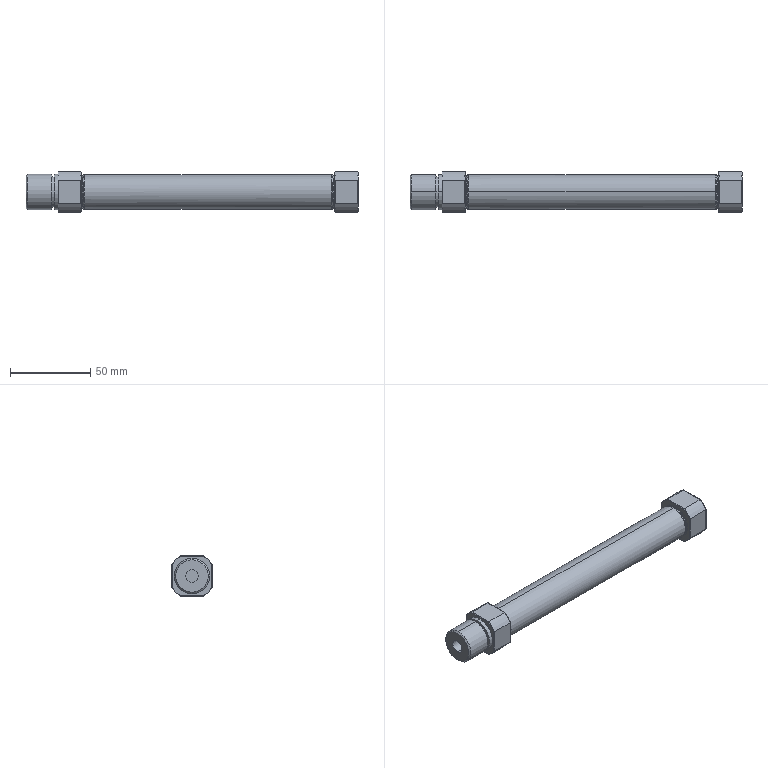Part | STEP file | _MI 20x125-S-U_c | 1 solid | 104 faces | box 207 x 25 x 25 mm | volume 36262 mm3 | cylinder 44 | spline 24 | plane 22 | cone 14 | commonest cylinder face diameters 0.6 x16 29 x8 21.4 x6 8.566 x4 22 x4 8 x2